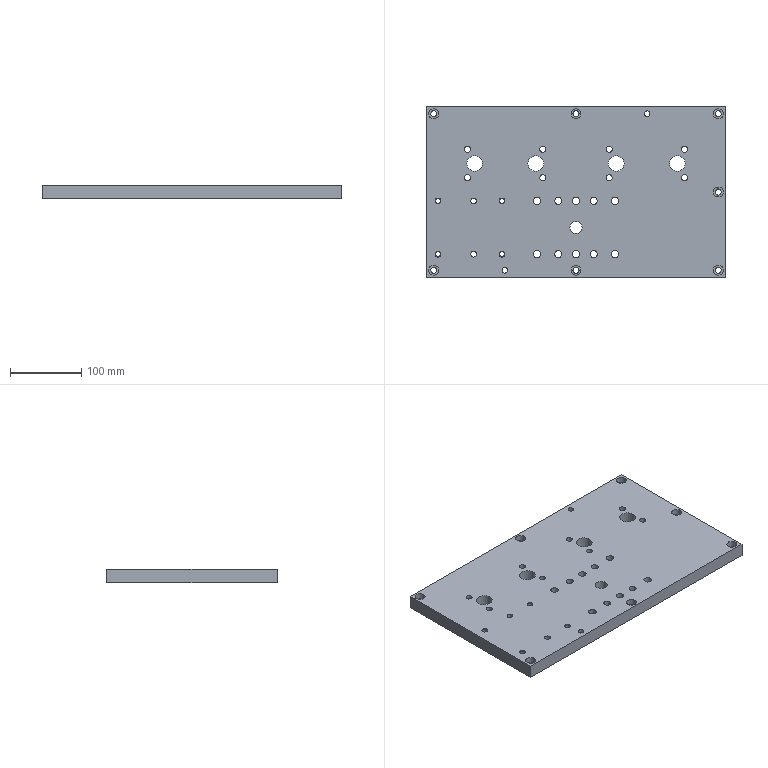Part | STEP file | Tube feed_id894_x_t | 1 solid | 94 faces | box 420 x 240 x 19.3 mm | volume 1848143 mm3 | cylinder 59 | plane 27 | cone 8 | commonest cylinder face diameters 8.5 x15 14 x15 10.6 x6 18 x6 6.8 x4 8 x4